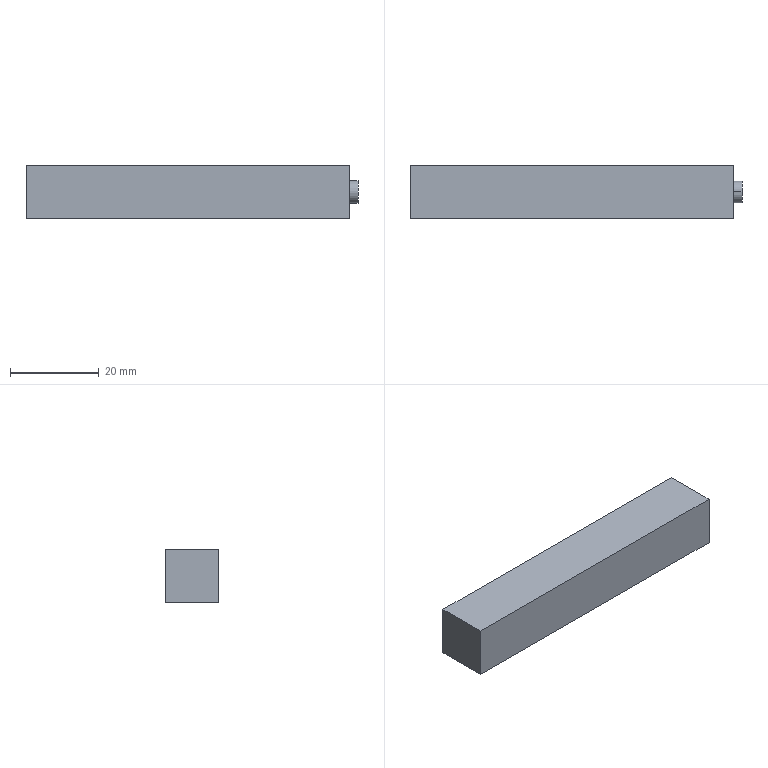Part | SolidWorks | features Extrusion 1, ICE 1 | 1 solid | 9 faces | box 75 x 12 x 12 mm | volume 10551 mm3 | plane 7 | cylinder 2 | commonest cylinder face diameters 5 x2
STEP:
#1=CARTESIAN_POINT('',(35.5,0.,3.5));
#2=VERTEX_POINT('',#1);
#3=CARTESIAN_POINT('',(35.5,0.,8.5));
#4=VERTEX_POINT('',#3);
#5=CARTESIAN_POINT('',(35.5,0.,6.));
#6=DIRECTION('',(1.,0.,0.));
#7=DIRECTION('',(0.,0.,-1.));
#8=AXIS2_PLACEMENT_3D('',#5,#6,#7);
#9=CIRCLE('',#8,2.5);
#10=EDGE_CURVE('',#2,#4,#9,.T.);
#11=ORIENTED_EDGE('',*,*,#10,.T.);
#12=CARTESIAN_POINT('',(37.5,0.,8.5));
#13=VERTEX_POINT('',#12);
#14=CARTESIAN_POINT('',(35.5,0.,8.5));
#15=DIRECTION('',(1.,0.,0.));
#16=VECTOR('',#15,1000.);
#17=LINE('',#14,#16);
#18=EDGE_CURVE('',#4,#13,#17,.T.);
#19=ORIENTED_EDGE('',*,*,#18,.T.);
#20=CARTESIAN_POINT('',(37.5,0.,3.5));
#21=VERTEX_POINT('',#20);
#22=CARTESIAN_POINT('',(37.5,0.,6.));
#23=DIRECTION('',(1.,0.,0.));
#24=DIRECTION('',(0.,0.,-1.));
#25=AXIS2_PLACEMENT_3D('',#22,#23,#24);
#26=CIRCLE('',#25,2.5);
#27=EDGE_CURVE('',#21,#13,#26,.T.);
#28=ORIENTED_EDGE('',*,*,#27,.F.);
#29=CARTESIAN_POINT('',(35.5,0.,3.5));
#30=DIRECTION('',(1.,0.,0.));
#31=VECTOR('',#30,1000.);
#32=LINE('',#29,#31);
#33=EDGE_CURVE('',#2,#21,#32,.T.);
#34=ORIENTED_EDGE('',*,*,#33,.F.);
#35=EDGE_LOOP('',(#11,#19,#28,#34));
#36=FACE_OUTER_BOUND('',#35,.T.);
#37=CARTESIAN_POINT('',(35.5,0.,6.));
#38=DIRECTION('',(1.,0.,0.));
#39=DIRECTION('',(0.,0.,-1.));
#40=AXIS2_PLACEMENT_3D('',#37,#38,#39);
#41=CYLINDRICAL_SURFACE('',#40,2.5);
#42=ADVANCED_FACE('',(#36),#41,.T.);
#43=CARTESIAN_POINT('',(35.5,6.,0.));
#44=VERTEX_POINT('',#43);
#45=CARTESIAN_POINT('',(35.5,6.,12.));
#46=VERTEX_POINT('',#45);
#47=CARTESIAN_POINT('',(35.5,6.,12.));
#48=DIRECTION('',(0.,0.,1.));
#49=VECTOR('',#48,1000.);
#50=LINE('',#47,#49);
#51=EDGE_CURVE('',#44,#46,#50,.T.);
#52=ORIENTED_EDGE('',*,*,#51,.F.);
#53=CARTESIAN_POINT('',(-37.5,6.,0.));
#54=VERTEX_POINT('',#53);
#55=CARTESIAN_POINT('',(-37.5,6.,0.));
#56=DIRECTION('',(-1.,0.,0.));
#57=VECTOR('',#56,1000.);
#58=LINE('',#55,#57);
#59=EDGE_CURVE('',#44,#54,#58,.T.);
#60=ORIENTED_EDGE('',*,*,#59,.T.);
#61=CARTESIAN_POINT('',(-37.5,6.,12.));
#62=VERTEX_POINT('',#61);
#63=CARTESIAN_POINT('',(-37.5,6.,12.));
#64=DIRECTION('',(0.,0.,-1.));
#65=VECTOR('',#64,1000.);
#66=LINE('',#63,#65);
#67=EDGE_CURVE('',#62,#54,#66,.T.);
#68=ORIENTED_EDGE('',*,*,#67,.F.);
#69=CARTESIAN_POINT('',(-37.5,6.,12.));
#70=DIRECTION('',(-1.,0.,0.));
#71=VECTOR('',#70,1000.);
#72=LINE('',#69,#71);
#73=EDGE_CURVE('',#46,#62,#72,.T.);
#74=ORIENTED_EDGE('',*,*,#73,.F.);
#75=EDGE_LOOP('',(#52,#60,#68,#74));
#76=FACE_OUTER_BOUND('',#75,.T.);
#77=CARTESIAN_POINT('',(-37.5,6.,12.));
#78=DIRECTION('',(0.,-1.,0.));
#79=DIRECTION('',(0.,0.,-1.));
#80=AXIS2_PLACEMENT_3D('',#77,#78,#79);
#81=PLANE('',#80);
#82=ADVANCED_FACE('',(#76),#81,.F.);
#83=CARTESIAN_POINT('',(35.5,-6.,12.));
#84=VERTEX_POINT('',#83);
#85=CARTESIAN_POINT('',(35.5,-6.,0.));
#86=VERTEX_POINT('',#85);
#87=CARTESIAN_POINT('',(35.5,-6.,12.));
#88=DIRECTION('',(0.,0.,-1.));
#89=VECTOR('',#88,1000.);
#90=LINE('',#87,#89);
#91=EDGE_CURVE('',#84,#86,#90,.T.);
#92=ORIENTED_EDGE('',*,*,#91,.F.);
#93=CARTESIAN_POINT('',(-37.5,-6.,12.));
#94=VERTEX_POINT('',#93);
#95=CARTESIAN_POINT('',(-37.5,-6.,12.));
#96=DIRECTION('',(1.,0.,0.));
#97=VECTOR('',#96,1000.);
#98=LINE('',#95,#97);
#99=EDGE_CURVE('',#94,#84,#98,.T.);
#100=ORIENTED_EDGE('',*,*,#99,.F.);
#101=CARTESIAN_POINT('',(-37.5,-6.,0.));
#102=VERTEX_POINT('',#101);
#103=CARTESIAN_POINT('',(-37.5,-6.,12.));
#104=DIRECTION('',(0.,0.,-1.));
#105=VECTOR('',#104,1000.);
#106=LINE('',#103,#105);
#107=EDGE_CURVE('',#94,#102,#106,.T.);
#108=ORIENTED_EDGE('',*,*,#107,.T.);
#109=CARTESIAN_POINT('',(-37.5,-6.,0.));
#110=DIRECTION('',(1.,0.,0.));
#111=VECTOR('',#110,1000.);
#112=LINE('',#109,#111);
#113=EDGE_CURVE('',#102,#86,#112,.T.);
#114=ORIENTED_EDGE('',*,*,#113,.T.);
#115=EDGE_LOOP('',(#92,#100,#108,#114));
#116=FACE_OUTER_BOUND('',#115,.T.);
#117=CARTESIAN_POINT('',(-37.5,-6.,12.));
#118=DIRECTION('',(0.,1.,0.));
#119=DIRECTION('',(0.,0.,1.));
#120=AXIS2_PLACEMENT_3D('',#117,#118,#119);
#121=PLANE('',#120);
#122=ADVANCED_FACE('',(#116),#121,.F.);
#123=ORIENTED_EDGE('',*,*,#99,.T.);
#124=CARTESIAN_POINT('',(35.5,0.,12.));
#125=DIRECTION('',(0.,1.,0.));
#126=VECTOR('',#125,1000.);
#127=LINE('',#124,#126);
#128=EDGE_CURVE('',#84,#46,#127,.T.);
#129=ORIENTED_EDGE('',*,*,#128,.T.);
#130=ORIENTED_EDGE('',*,*,#73,.T.);
#131=CARTESIAN_POINT('',(-37.5,6.,12.));
#132=DIRECTION('',(0.,-1.,0.));
#133=VECTOR('',#132,1000.);
#134=LINE('',#131,#133);
#135=EDGE_CURVE('',#62,#94,#134,.T.);
#136=ORIENTED_EDGE('',*,*,#135,.T.);
#137=EDGE_LOOP('',(#123,#129,#130,#136));
#138=FACE_OUTER_BOUND('',#137,.T.);
#139=CARTESIAN_POINT('',(0.,0.,12.));
#140=DIRECTION('',(0.,0.,1.));
#141=DIRECTION('',(1.,0.,0.));
#142=AXIS2_PLACEMENT_3D('',#139,#140,#141);
#143=PLANE('',#142);
#144=ADVANCED_FACE('',(#138),#143,.T.);
#145=CARTESIAN_POINT('',(35.5,0.,0.));
#146=DIRECTION('',(0.,1.,0.));
#147=VECTOR('',#146,1000.);
#148=LINE('',#145,#147);
#149=EDGE_CURVE('',#86,#44,#148,.T.);
#150=ORIENTED_EDGE('',*,*,#149,.F.);
#151=ORIENTED_EDGE('',*,*,#113,.F.);
#152=CARTESIAN_POINT('',(-37.5,6.,0.));
#153=DIRECTION('',(0.,-1.,0.));
#154=VECTOR('',#153,1000.);
#155=LINE('',#152,#154);
#156=EDGE_CURVE('',#54,#102,#155,.T.);
#157=ORIENTED_EDGE('',*,*,#156,.F.);
#158=ORIENTED_EDGE('',*,*,#59,.F.);
#159=EDGE_LOOP('',(#150,#151,#157,#158));
#160=FACE_OUTER_BOUND('',#159,.T.);
#161=CARTESIAN_POINT('',(0.,0.,0.));
#162=DIRECTION('',(0.,0.,1.));
#163=DIRECTION('',(1.,0.,0.));
#164=AXIS2_PLACEMENT_3D('',#161,#162,#163);
#165=PLANE('',#164);
#166=ADVANCED_FACE('',(#160),#165,.F.);
#167=ORIENTED_EDGE('',*,*,#156,.T.);
#168=ORIENTED_EDGE('',*,*,#107,.F.);
#169=ORIENTED_EDGE('',*,*,#135,.F.);
#170=ORIENTED_EDGE('',*,*,#67,.T.);
#171=EDGE_LOOP('',(#167,#168,#169,#170));
#172=FACE_OUTER_BOUND('',#171,.T.);
#173=CARTESIAN_POINT('',(-37.5,6.,12.));
#174=DIRECTION('',(1.,0.,0.));
#175=DIRECTION('',(0.,0.,-1.));
#176=AXIS2_PLACEMENT_3D('',#173,#174,#175);
#177=PLANE('',#176);
#178=ADVANCED_FACE('',(#172),#177,.F.);
#179=ORIENTED_EDGE('',*,*,#91,.T.);
#180=ORIENTED_EDGE('',*,*,#149,.T.);
#181=ORIENTED_EDGE('',*,*,#51,.T.);
#182=ORIENTED_EDGE('',*,*,#128,.F.);
#183=EDGE_LOOP('',(#179,#180,#181,#182));
#184=FACE_OUTER_BOUND('',#183,.T.);
#185=ORIENTED_EDGE('',*,*,#10,.F.);
#186=CARTESIAN_POINT('',(35.5,0.,6.));
#187=DIRECTION('',(1.,0.,0.));
#188=DIRECTION('',(0.,0.,-1.));
#189=AXIS2_PLACEMENT_3D('',#186,#187,#188);
#190=CIRCLE('',#189,2.5);
#191=EDGE_CURVE('',#4,#2,#190,.T.);
#192=ORIENTED_EDGE('',*,*,#191,.F.);
#193=EDGE_LOOP('',(#185,#192));
#194=FACE_BOUND('',#193,.T.);
#195=CARTESIAN_POINT('',(35.5,0.,6.));
#196=DIRECTION('',(1.,0.,0.));
#197=DIRECTION('',(0.,0.,-1.));
#198=AXIS2_PLACEMENT_3D('',#195,#196,#197);
#199=PLANE('',#198);
#200=ADVANCED_FACE('',(#184,#194),#199,.T.);
#201=ORIENTED_EDGE('',*,*,#18,.F.);
#202=ORIENTED_EDGE('',*,*,#191,.T.);
#203=ORIENTED_EDGE('',*,*,#33,.T.);
#204=CARTESIAN_POINT('',(37.5,0.,6.));
#205=DIRECTION('',(1.,0.,0.));
#206=DIRECTION('',(0.,0.,-1.));
#207=AXIS2_PLACEMENT_3D('',#204,#205,#206);
#208=CIRCLE('',#207,2.5);
#209=EDGE_CURVE('',#13,#21,#208,.T.);
#210=ORIENTED_EDGE('',*,*,#209,.F.);
#211=EDGE_LOOP('',(#201,#202,#203,#210));
#212=FACE_OUTER_BOUND('',#211,.T.);
#213=CARTESIAN_POINT('',(35.5,0.,6.));
#214=DIRECTION('',(1.,0.,0.));
#215=DIRECTION('',(0.,0.,-1.));
#216=AXIS2_PLACEMENT_3D('',#213,#214,#215);
#217=CYLINDRICAL_SURFACE('',#216,2.5);
#218=ADVANCED_FACE('',(#212),#217,.T.);
#219=ORIENTED_EDGE('',*,*,#27,.T.);
#220=ORIENTED_EDGE('',*,*,#209,.T.);
#221=EDGE_LOOP('',(#219,#220));
#222=FACE_OUTER_BOUND('',#221,.T.);
#223=CARTESIAN_POINT('',(37.5,6.,12.));
#224=DIRECTION('',(-1.,0.,0.));
#225=DIRECTION('',(0.,0.,1.));
#226=AXIS2_PLACEMENT_3D('',#223,#224,#225);
#227=PLANE('',#226);
#228=ADVANCED_FACE('',(#222),#227,.F.);
#229=CLOSED_SHELL('',(#42,#82,#122,#144,#166,#178,#200,#218,#228));
#230=MANIFOLD_SOLID_BREP('',#229);
#231=CARTESIAN_POINT('',(0.,0.,0.));
#232=DIRECTION('',(0.,0.,1.));
#233=DIRECTION('',(1.,0.,0.));
#234=AXIS2_PLACEMENT_3D('',#231,#232,#233);
#235=(LENGTH_UNIT()NAMED_UNIT(*)SI_UNIT(.MILLI.,.METRE.));
#236=UNCERTAINTY_MEASURE_WITH_UNIT(LENGTH_MEASURE(0.00001),#235,'','');
#237=(NAMED_UNIT(*)PLANE_ANGLE_UNIT()SI_UNIT($,.RADIAN.));
#238=(NAMED_UNIT(*)SI_UNIT($,.STERADIAN.)SOLID_ANGLE_UNIT());
#239=(GEOMETRIC_REPRESENTATION_CONTEXT(3)GLOBAL_UNCERTAINTY_ASSIGNED_CONTEXT((#236))GLOBAL_UNIT_ASSIGNED_CONTEXT((#235,#237,#238))REPRESENTATION_CONTEXT('',''));
#240=ADVANCED_BREP_SHAPE_REPRESENTATION('',(#230,#234),#239);